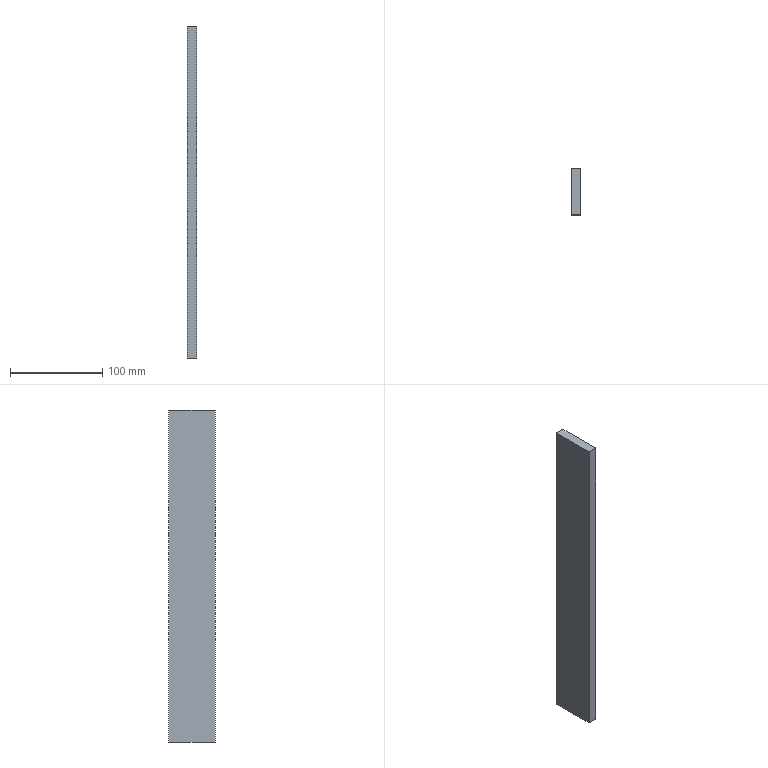Part | NX | features solid 2 | 1 solid | 6 faces | box 10 x 50 x 360 mm | volume 180000 mm3 | plane 6
STEP:
#1=CARTESIAN_POINT('',(-1605.,610.,245.));
#2=VERTEX_POINT('',#1);
#3=CARTESIAN_POINT('',(-1605.,560.,245.));
#4=VERTEX_POINT('',#3);
#5=CARTESIAN_POINT('',(-1605.,610.,245.));
#6=DIRECTION('',(0.,1.,0.));
#7=VECTOR('',#6,1000.);
#8=LINE('',#5,#7);
#9=EDGE_CURVE('',#2,#4,#8,.F.);
#10=ORIENTED_EDGE('',*,*,#9,.T.);
#11=CARTESIAN_POINT('',(-1605.,560.,-115.));
#12=VERTEX_POINT('',#11);
#13=CARTESIAN_POINT('',(-1605.,560.,175.));
#14=DIRECTION('',(0.,0.,-1.));
#15=VECTOR('',#14,1000.);
#16=LINE('',#13,#15);
#17=EDGE_CURVE('',#4,#12,#16,.T.);
#18=ORIENTED_EDGE('',*,*,#17,.T.);
#19=CARTESIAN_POINT('',(-1605.,610.,-115.));
#20=VERTEX_POINT('',#19);
#21=CARTESIAN_POINT('',(-1605.,610.,-115.));
#22=DIRECTION('',(0.,-1.,0.));
#23=VECTOR('',#22,1000.);
#24=LINE('',#21,#23);
#25=EDGE_CURVE('',#20,#12,#24,.T.);
#26=ORIENTED_EDGE('',*,*,#25,.F.);
#27=CARTESIAN_POINT('',(-1605.,610.,175.));
#28=DIRECTION('',(0.,0.,-1.));
#29=VECTOR('',#28,1000.);
#30=LINE('',#27,#29);
#31=EDGE_CURVE('',#2,#20,#30,.T.);
#32=ORIENTED_EDGE('',*,*,#31,.F.);
#33=EDGE_LOOP('',(#10,#18,#26,#32));
#34=FACE_BOUND('',#33,.T.);
#35=CARTESIAN_POINT('',(-1605.,610.,175.));
#36=DIRECTION('',(1.,0.,0.));
#37=DIRECTION('',(0.,0.,-1.));
#38=AXIS2_PLACEMENT_3D('',#35,#36,#37);
#39=PLANE('',#38);
#40=ADVANCED_FACE('',(#34),#39,.T.);
#41=ORIENTED_EDGE('',*,*,#25,.T.);
#42=CARTESIAN_POINT('',(-1615.,560.,-115.));
#43=VERTEX_POINT('',#42);
#44=CARTESIAN_POINT('',(-1605.,560.,-115.));
#45=DIRECTION('',(1.,0.,0.));
#46=VECTOR('',#45,1000.);
#47=LINE('',#44,#46);
#48=EDGE_CURVE('',#12,#43,#47,.F.);
#49=ORIENTED_EDGE('',*,*,#48,.T.);
#50=CARTESIAN_POINT('',(-1615.,610.,-115.));
#51=VERTEX_POINT('',#50);
#52=CARTESIAN_POINT('',(-1615.,610.,-115.));
#53=DIRECTION('',(0.,1.,0.));
#54=VECTOR('',#53,1000.);
#55=LINE('',#52,#54);
#56=EDGE_CURVE('',#51,#43,#55,.F.);
#57=ORIENTED_EDGE('',*,*,#56,.F.);
#58=CARTESIAN_POINT('',(-1605.,610.,-115.));
#59=DIRECTION('',(1.,0.,0.));
#60=VECTOR('',#59,1000.);
#61=LINE('',#58,#60);
#62=EDGE_CURVE('',#20,#51,#61,.F.);
#63=ORIENTED_EDGE('',*,*,#62,.F.);
#64=EDGE_LOOP('',(#41,#49,#57,#63));
#65=FACE_BOUND('',#64,.T.);
#66=CARTESIAN_POINT('',(-1605.,610.,-115.));
#67=DIRECTION('',(0.,0.,-1.));
#68=DIRECTION('',(-1.,0.,0.));
#69=AXIS2_PLACEMENT_3D('',#66,#67,#68);
#70=PLANE('',#69);
#71=ADVANCED_FACE('',(#65),#70,.T.);
#72=ORIENTED_EDGE('',*,*,#56,.T.);
#73=CARTESIAN_POINT('',(-1615.,560.,245.));
#74=VERTEX_POINT('',#73);
#75=CARTESIAN_POINT('',(-1615.,560.,175.));
#76=DIRECTION('',(0.,0.,-1.));
#77=VECTOR('',#76,1000.);
#78=LINE('',#75,#77);
#79=EDGE_CURVE('',#74,#43,#78,.T.);
#80=ORIENTED_EDGE('',*,*,#79,.F.);
#81=CARTESIAN_POINT('',(-1615.,610.,245.));
#82=VERTEX_POINT('',#81);
#83=CARTESIAN_POINT('',(-1615.,610.,245.));
#84=DIRECTION('',(0.,-1.,0.));
#85=VECTOR('',#84,1000.);
#86=LINE('',#83,#85);
#87=EDGE_CURVE('',#82,#74,#86,.T.);
#88=ORIENTED_EDGE('',*,*,#87,.F.);
#89=CARTESIAN_POINT('',(-1615.,610.,175.));
#90=DIRECTION('',(0.,0.,-1.));
#91=VECTOR('',#90,1000.);
#92=LINE('',#89,#91);
#93=EDGE_CURVE('',#82,#51,#92,.T.);
#94=ORIENTED_EDGE('',*,*,#93,.T.);
#95=EDGE_LOOP('',(#72,#80,#88,#94));
#96=FACE_BOUND('',#95,.T.);
#97=CARTESIAN_POINT('',(-1615.,610.,175.));
#98=DIRECTION('',(1.,0.,0.));
#99=DIRECTION('',(0.,0.,-1.));
#100=AXIS2_PLACEMENT_3D('',#97,#98,#99);
#101=PLANE('',#100);
#102=ADVANCED_FACE('',(#96),#101,.F.);
#103=CARTESIAN_POINT('',(-1605.,610.,245.));
#104=DIRECTION('',(-1.,0.,0.));
#105=VECTOR('',#104,1000.);
#106=LINE('',#103,#105);
#107=EDGE_CURVE('',#2,#82,#106,.T.);
#108=ORIENTED_EDGE('',*,*,#107,.T.);
#109=ORIENTED_EDGE('',*,*,#87,.T.);
#110=CARTESIAN_POINT('',(-1605.,560.,245.));
#111=DIRECTION('',(-1.,0.,0.));
#112=VECTOR('',#111,1000.);
#113=LINE('',#110,#112);
#114=EDGE_CURVE('',#4,#74,#113,.T.);
#115=ORIENTED_EDGE('',*,*,#114,.F.);
#116=ORIENTED_EDGE('',*,*,#9,.F.);
#117=EDGE_LOOP('',(#108,#109,#115,#116));
#118=FACE_BOUND('',#117,.T.);
#119=CARTESIAN_POINT('',(-1605.,610.,245.));
#120=DIRECTION('',(0.,0.,-1.));
#121=DIRECTION('',(-1.,0.,0.));
#122=AXIS2_PLACEMENT_3D('',#119,#120,#121);
#123=PLANE('',#122);
#124=ADVANCED_FACE('',(#118),#123,.F.);
#125=ORIENTED_EDGE('',*,*,#79,.T.);
#126=ORIENTED_EDGE('',*,*,#48,.F.);
#127=ORIENTED_EDGE('',*,*,#17,.F.);
#128=ORIENTED_EDGE('',*,*,#114,.T.);
#129=EDGE_LOOP('',(#125,#126,#127,#128));
#130=FACE_BOUND('',#129,.T.);
#131=CARTESIAN_POINT('',(-1605.,560.,175.));
#132=DIRECTION('',(0.,1.,0.));
#133=DIRECTION('',(0.,0.,-1.));
#134=AXIS2_PLACEMENT_3D('',#131,#132,#133);
#135=PLANE('',#134);
#136=ADVANCED_FACE('',(#130),#135,.F.);
#137=ORIENTED_EDGE('',*,*,#93,.F.);
#138=ORIENTED_EDGE('',*,*,#107,.F.);
#139=ORIENTED_EDGE('',*,*,#31,.T.);
#140=ORIENTED_EDGE('',*,*,#62,.T.);
#141=EDGE_LOOP('',(#137,#138,#139,#140));
#142=FACE_BOUND('',#141,.T.);
#143=CARTESIAN_POINT('',(-1605.,610.,175.));
#144=DIRECTION('',(0.,1.,0.));
#145=DIRECTION('',(0.,0.,-1.));
#146=AXIS2_PLACEMENT_3D('',#143,#144,#145);
#147=PLANE('',#146);
#148=ADVANCED_FACE('',(#142),#147,.T.);
#149=CLOSED_SHELL('',(#40,#71,#102,#124,#136,#148));
#150=MANIFOLD_SOLID_BREP('',#149);
#151=(LENGTH_UNIT()NAMED_UNIT(*)SI_UNIT(.MILLI.,.METRE.));
#152=UNCERTAINTY_MEASURE_WITH_UNIT(LENGTH_MEASURE(0.00001),#151,'','');
#153=(NAMED_UNIT(*)PLANE_ANGLE_UNIT()SI_UNIT($,.RADIAN.));
#154=(NAMED_UNIT(*)SI_UNIT($,.STERADIAN.)SOLID_ANGLE_UNIT());
#155=(GEOMETRIC_REPRESENTATION_CONTEXT(3)GLOBAL_UNCERTAINTY_ASSIGNED_CONTEXT((#152))GLOBAL_UNIT_ASSIGNED_CONTEXT((#151,#153,#154))REPRESENTATION_CONTEXT('',''));
#156=ADVANCED_BREP_SHAPE_REPRESENTATION('',(#150),#155);